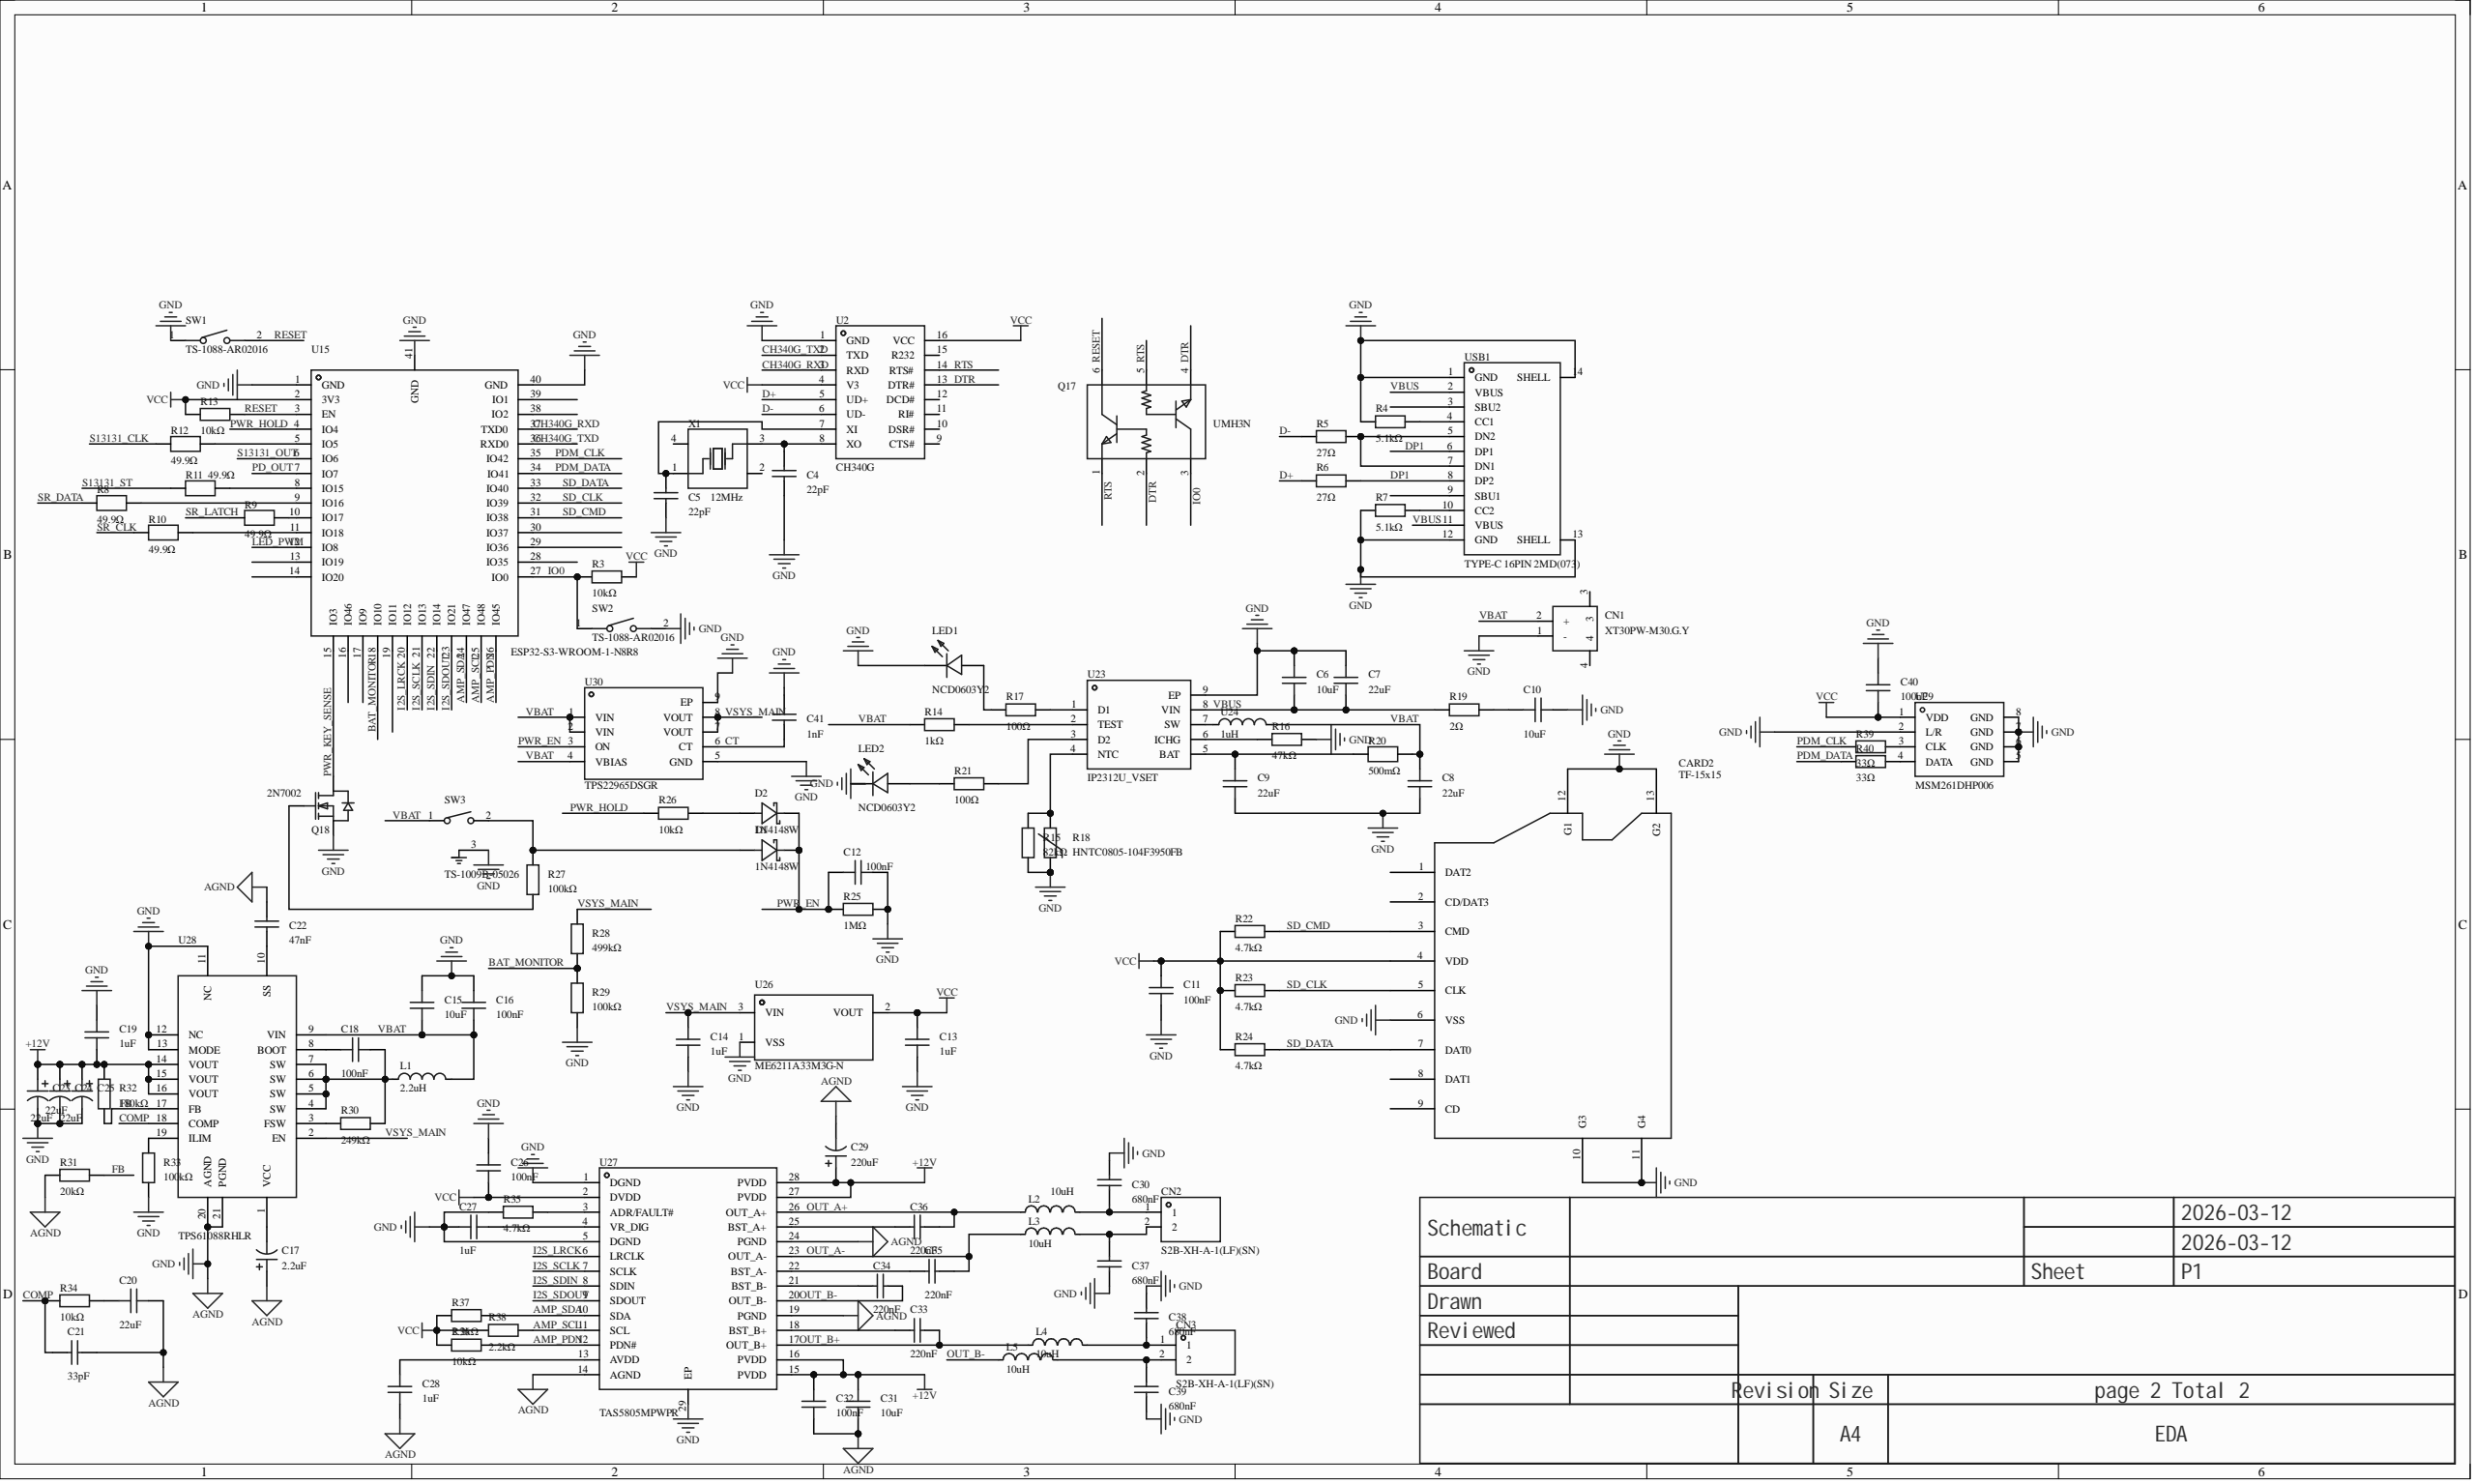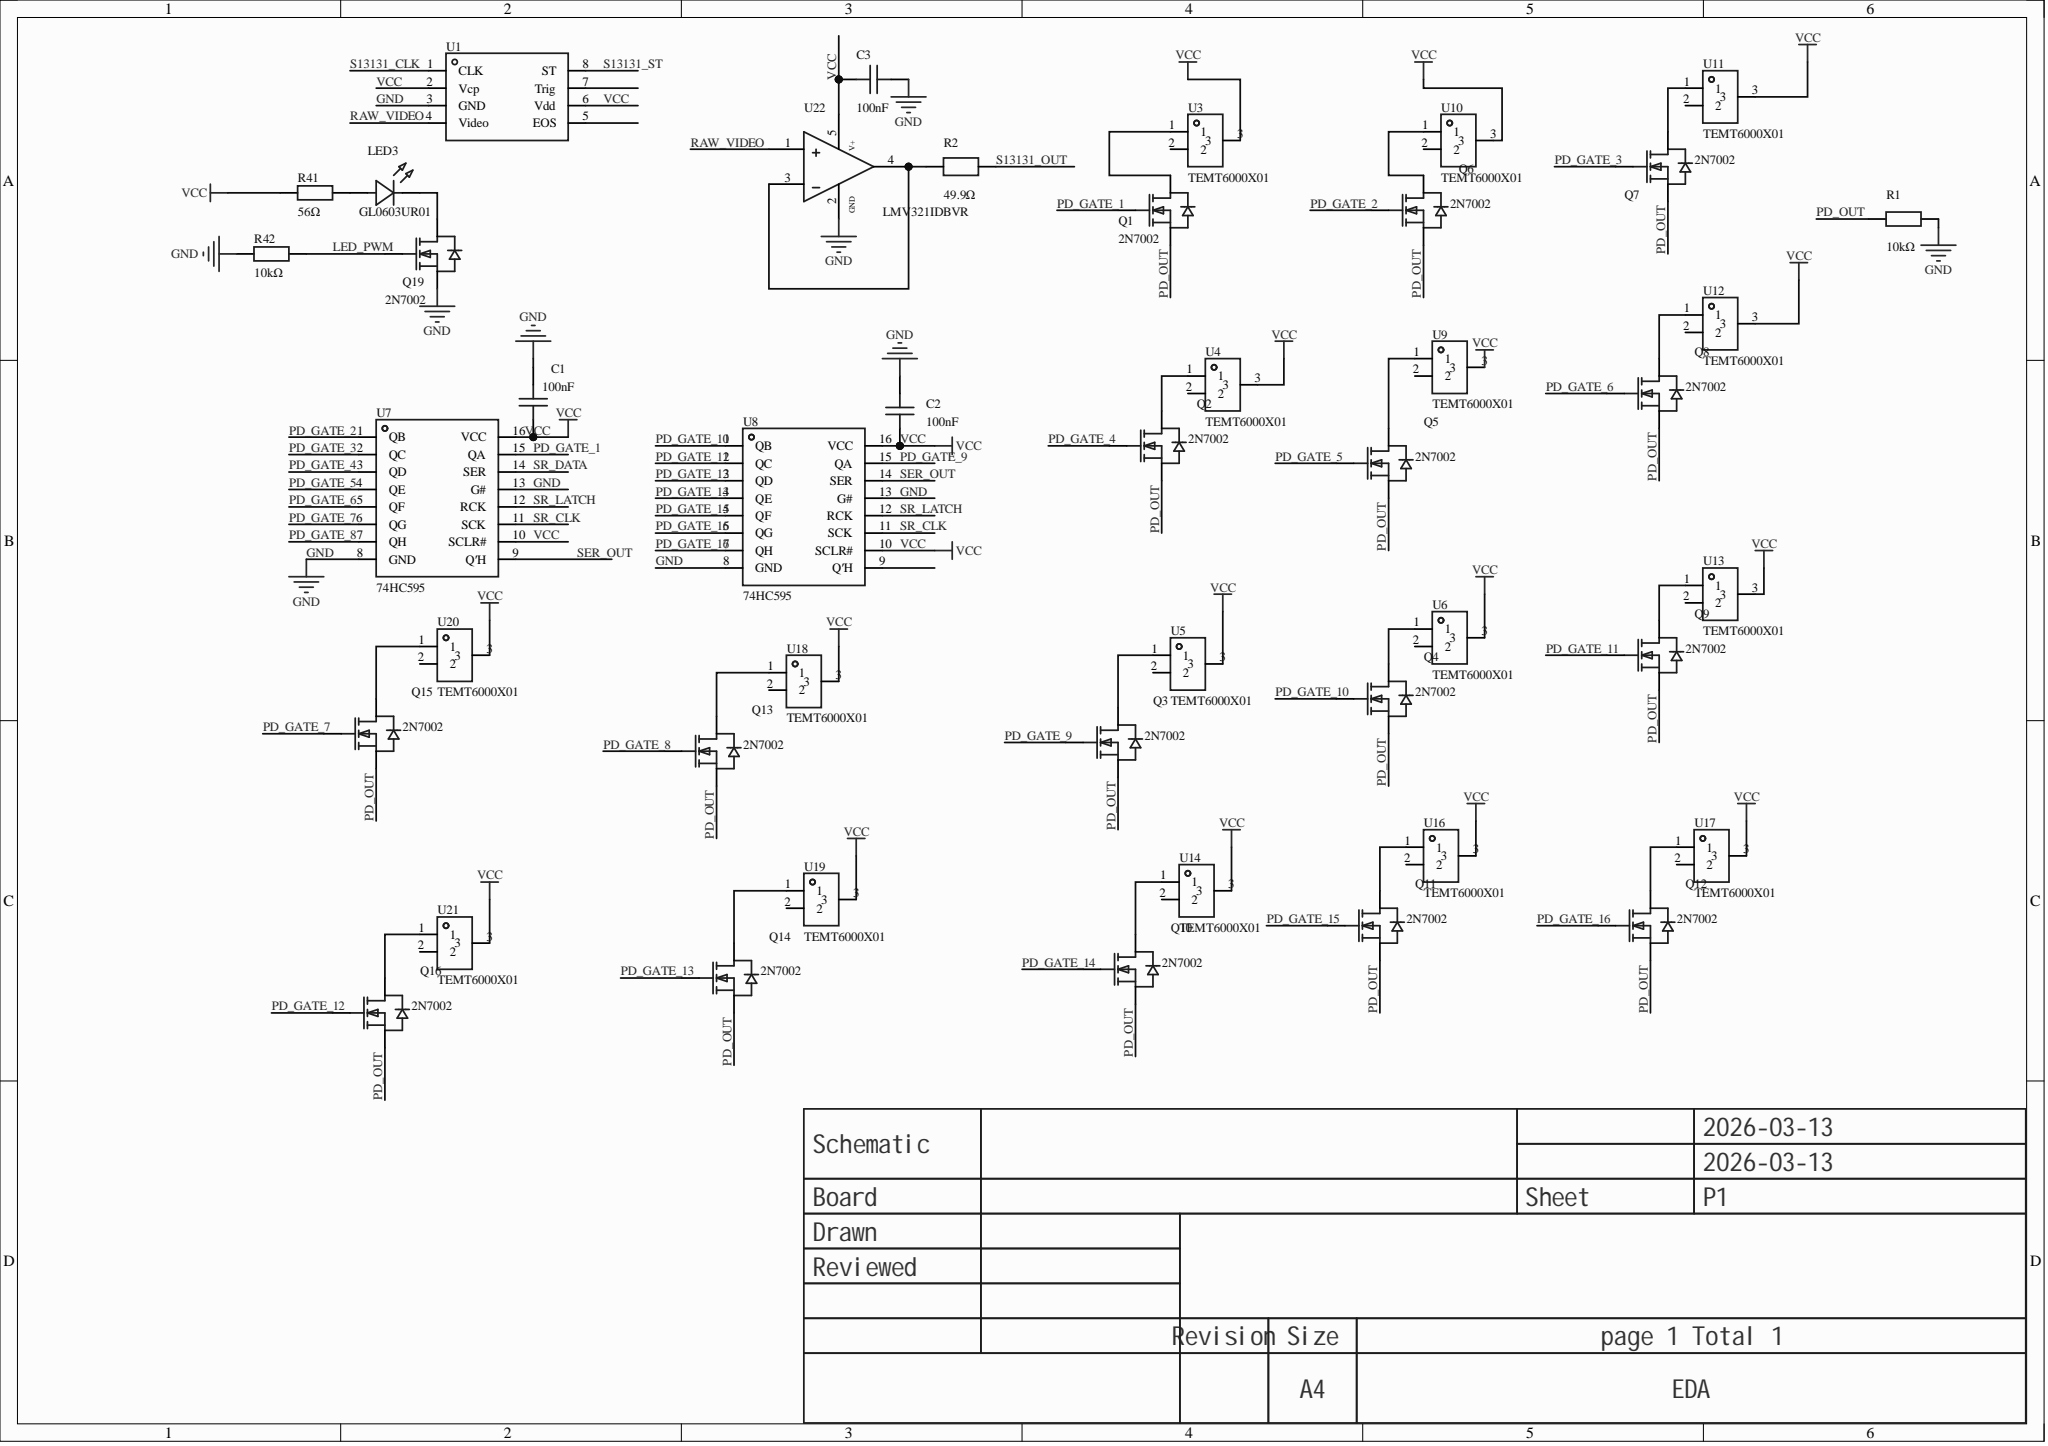Circuit board | Altium Designer | 150 parts | 126 nets
Bill of materials:
Comment,Description,Designator,Footprint,LibRef,Quantity
"100nF","Capacitance: 100nF; Tolerance: ±10%; Rated voltage: 50V; Temp. coefficient: X7R;","C1, C2, C3, C11, C12, C16, C18, C26, C32, C40","C0603","CGA0603X7R104K500JT","10"
"22pF","Capacitance: 22pF; Tolerance: ±5%; Rated voltage: 50V; Temp. coefficient: C0G;","C4, C5","C0603","CL10C220JB8NNNC","2"
"10uF","Capacitance: 10uF; Tolerance: ±20%; Rated voltage: 25V; Temp. coefficient: X5R;","C6, C10, C15, C31","C0603","CL10A106MA8NRNC","4"
"22uF","Capacitance: 22uF; Tolerance: ±20%; Rated voltage: 16V; Temp. coefficient: X5R;","C7, C8, C9, C20","C0603","CGA0603X5R226M160JT","4"
"1uF","Capacitance: 1uF; Tolerance: ±10%; Rated voltage: 50V; Temp. coefficient: X5R;","C13, C14, C19, C27, C28","C0603","CL10A105KB8NNNC","5"
"2.2uF","Capacitance: 2.2uF; Tolerance: ±20%; Rated voltage: 50V; Type: Polymer;","C17","CAP-SMD_BD5.0-L5.3-W5.3-LS6.0-FD","RYHV50V2.2UF5*5","1"
"33pF","Capacitance: 33pF; Tolerance: ±5%; Rated voltage: 50V; Temp. coefficient: C0G;","C21","C0603","CL10C330JB8NNNC","1"
"47nF","Capacitance: 47nF; Tolerance: ±10%; Rated voltage: 50V; Temp. coefficient: X7R;","C22","C0603","CL10B473KB8NNNC","1"
"22uF","Capacitance: 22uF; Tolerance: ±20%; Rated voltage: 25V; Ripple current: 26mA@120Hz;","C23, C24, C25","CAP-SMD_BD5.0-L5.3-W5.3-LS6.3-FD-1","RVT25V22M5X5","3"
"220uF","Capacitance: 220uF; Tolerance: ±20%; Rated voltage: 25V; Ripple current: 120mA@120Hz;","C29","CAP-SMD_BD6.3-L6.6-W6.6-LS7.3-FD-H7.7","JVJ25V220M6x8","1"
"680nF","Capacitance: 680nF; Tolerance: ±10%; Rated voltage: 16V; Temp. coefficient: X7R;","C30, C37, C38, C39","C0603","CC0603KRX7R7BB684","4"
"220nF","Capacitance: 220nF; Tolerance: ±10%; Rated voltage: 25V; Temp. coefficient: X7R;","C33, C34, C35, C36","C0603","CL10B224KA8NNNC","4"
"1nF","Capacitance: 1nF; Tolerance: ±10%; Rated voltage: 50V; Temp. coefficient: X7R;","C41","C0603","CL10B102KB8NNNC","1"
"TF-15x15","Card connection: Self-ejecting; Card type: MicroSD card (TF card); Connector type: Socket; Max body height: 2mm; Operating temp.: -25℃~+85℃;","CARD2","TF-SMD_TF-15-15","TF-15x15","1"
"XT30PW-M30.G.Y","Socket,DCsupply,XT30,male,PIN:2","CN1","CONN-TH_XT30PW-M","XT30PW-M30.G.Y","1"
"S2B-XH-A-1(LF)(SN)","Pin structure: 1x2P; Pitch: 2.5mm; Mounting: Right-angle THT; Series: XH; Total pins: 2P; Rows: 1; Pins per row: 2; Row spacing: -; Rated current: 3A; Contact material: Brass; Contact plating: Tin; Operating temp.: -25℃~+85℃;","CN2, CN3","CONN-TH_S2B-XH-A-1-LF-SN","S2B-XH-A-1(LF)(SN)","2"
"1N4148W","Diode configuration: Discrete; Forward voltage drop (Vf): 1.25V@150mA; DC reverse voltage (Vr): 100V; Rectified current: 150mA; Reverse recovery time (Trr): 4ns;","D1, D2","SOD-123_L2.7-W1.6-LS3.7-FD","1N4148W_C7420318","2"
"2.2uH","Inductance: 2.2uH; Tolerance: ±20%; Rated current: 4A; Saturation current (Isat): 5A; Type: Molded inductor;","L1","IND-SMD_L4.6-W4.1_MHCI04015","SRG0420-2R2-M","1"
"10uH","Inductance: 10uH; Tolerance: ±20%; Rated current: 4.5A; Saturation current (Isat): 5.5A; Type: Molded inductor;","L2, L3, L4, L5","IND-SMD_L7.3-W6.8","FXL0630-100-M","4"
"NCD0603Y2","Emitted color: Yellow; Forward voltage (VF): 1.6V~2.6V; Power: 65mW; Forward current: 20mA; Dominant wavelength: 586nm~595nm; Lens color: Clear lens; Luminous intensity: 100mcd~220mcd; Viewing angle: 130°; Operating temp.: -30℃~+85℃;","LED1, LED2","LED0603-RD","NCD0603Y2","2"
"GL0603UR01","Emitted color: Red; Forward voltage (Vf): 2.4V; Forward current: 20mA; Wavelength: 620nm~625nm; Diode configuration: Discrete diode; Lens color: Clear lens; Luminous intensity: 120mcd; Viewing angle: 120°; Tape mount: Top SMD; Operating temp.: -40℃~+85℃;","LED3","LED0603-FD","GL0603UR01","1"
"2N7002","Quantity: 1 N-channel; Drain-source voltage (Vdss): 60V; Continuous drain current (Id): 115mA; On-resistance (RDS(on)): 5Ω@10V; Power dissipation (Pd): 225mW; Threshold voltage (Vgs(th)): 2.5V;","Q1, Q2, Q3, Q4, Q5, Q6, Q7, Q8, Q9, Q10, Q11, Q12, Q13, Q14, Q15, Q16, Q18, Q19","SOT-23-3_L2.9-W1.3-P1.90-LS2.4-BR","2N7002_C8545","18"
"UMH3N","Quantity: -; Collector-emitter breakdown voltage (Vceo): 50V; Collector current (Ic): 100mA; Power dissipation (Pd): 150mW; DC current gain (hFE): 100@1mA,5V;","Q17","SC-70-6_L2.2-W1.3-P0.65-LS2.1-BR","UMH3N","1"
"10kΩ","Resistor type: Thick-film; Resistance: 10kΩ; Tolerance: ±1%; Power: 100mW; Working voltage: 75V; Temp. coefficient: ±100ppm/?;","R1, R3, R13, R26, R34, R36, R42","R0603","0603WAF1002T5E","7"
"49.9Ω","Resistor type: Thick-film; Resistance: 49.9Ω; Tolerance: ±1%; Power: 100mW; Working voltage: 75V; Temp. coefficient: ±100ppm/?;","R2, R8, R9, R10, R11, R12","R0603","FRC0603F49R9TS","6"
"5.1kΩ","Resistor type: Thick-film; Resistance: 5.1kΩ; Tolerance: ±1%; Power: 100mW; Working voltage: 75V; Temp. coefficient: ±100ppm/?;","R4, R7","R0603","0603WAF5101T5E","2"
"27Ω","Resistor type: Thick-film; Resistance: 27Ω; Tolerance: ±1%; Power: 100mW; Working voltage: 75V; Temp. coefficient: ±200ppm/?;","R5, R6","R0603","0603WAF270JT5E","2"
"1kΩ","Resistor type: Thick-film; Resistance: 1kΩ; Tolerance: ±1%; Power: 100mW; Working voltage: 75V; Temp. coefficient: ±100ppm/?;","R14","R0603","0603WAF1001T5E","1"
"82kΩ","Resistor type: Thick-film; Resistance: 82kΩ; Tolerance: ±1%; Power: 100mW; Working voltage: 75V; Temp. coefficient: ±100ppm/?;","R15","R0603","0603WAF8202T5E","1"
"47kΩ","Resistor type: Thick-film; Resistance: 47kΩ; Tolerance: ±1%; Power: 100mW; Working voltage: 75V; Temp. coefficient: ±100ppm/?;","R16","R0603","0603WAF4702T5E","1"
"100Ω","Resistor type: Thick-film; Resistance: 100Ω; Tolerance: ±1%; Power: 100mW; Max working voltage: 75V; Temp. coefficient: ±200ppm/?;","R17, R21","R0603","0603WAF1000T5E","2"
"HNTC0805-104F3950FB","","R18","R0805","HNTC0805-104F3950FB","1"
"2Ω","Resistor type: Thick-film; Resistance: 2Ω; Tolerance: ±1%; Power: 100mW; Max working voltage: 75V; Temp. coefficient: ±200ppm/?;","R19","R0603","RC0603FR-072RL","1"
"500mΩ","Resistor type: Thin-film; Resistance: 500mΩ; Tolerance: ±1%; Power: 1W; Temp. coefficient: ±100ppm/?;","R20","R1206","HoJLRH1206-1W-500mR-1%","1"
"4.7kΩ","Resistor type: Thick-film; Resistance: 4.7kΩ; Tolerance: ±1%; Power: 100mW; Working voltage: 75V; Temp. coefficient: ±100ppm/?;","R22, R23, R24, R35","R0603","0603WAF4701T5E","4"
"1MΩ","Resistor type: Thick-film; Resistance: 1MΩ; Tolerance: ±1%; Power: 100mW; Max working voltage: 75V; Temp. coefficient: ±100ppm/?;","R25","R0603","0603WAF1004T5E","1"
"100kΩ","Resistor type: Thick-film; Resistance: 100kΩ; Tolerance: ±1%; Power: 100mW; Working voltage: 75V; Temp. coefficient: ±100ppm/?;","R27, R29, R33","R0603","0603WAF1003T5E","3"
"499kΩ","Resistor type: Thick-film; Resistance: 499kΩ; Tolerance: ±1%; Power: 100mW; Working voltage: 75V; Temp. coefficient: ±100ppm/?;","R28","R0603","0603WAF4993T5E","1"
"249kΩ","Resistor type: Thick-film; Resistance: 249kΩ; Tolerance: ±1%; Power: 100mW; Working voltage: 75V; Temp. coefficient: ±100ppm/?;","R30","R0603","0603WAF2493T5E","1"
"20kΩ","Resistor type: Thick-film; Resistance: 20kΩ; Tolerance: ±1%; Power: 100mW; Working voltage: 75V; Temp. coefficient: ±100ppm/?;","R31","R0603","0603WAF2002T5E","1"
"180kΩ","Resistor type: Thick-film; Resistance: 180kΩ; Tolerance: ±1%; Power: 100mW; Working voltage: 75V; Temp. coefficient: ±100ppm/?;","R32","R0603","0603WAF1803T5E","1"
"2.2kΩ","Resistor type: Thick-film; Resistance: 2.2kΩ; Tolerance: ±1%; Power: 100mW; Max working voltage: 75V; Temp. coefficient: ±100ppm/?;","R37, R38","R0603","0603WAF2201T5E","2"
"33Ω","Resistor type: Thick-film; Resistance: 33Ω; Tolerance: ±1%; Power: 100mW; Working voltage: 75V; Temp. coefficient: ±100ppm/?;","R39, R40","R0603","0603WAF330JT5E","2"
"56Ω","Resistor type: Thick-film; Resistance: 56Ω; Tolerance: ±1%; Power: 100mW; Max working voltage: 75V; Temp. coefficient: ±200ppm/?;","R41","R0603","0603WAF560JT5E","1"
"TS-1088-AR02016","Circuit: SPST; Button shape: Round; Actuating force: 1.6N; Mounting: Upright SMD; Switch length: 4mm; Switch width: 3mm; Switch height: 2mm; Bracket: Without bracket; Contact current: 50mA; Rated voltage: 12V; Life: 10万 cycles;","SW1, SW2","SW-SMD_L3.9-W3.0-P4.45","TS-1088-AR02016","2"
"TS-1009B-05026","Circuit: SPST; Button shape: Round; Mounting: Right-angle THT; Switch length: 4.5mm; Switch width: 4.5mm; Switch height: 5mm; Contact current: 50mA; Rated voltage: 12V; LED: -; Life: -;","SW3","SW-TH_3P-L4.5-W3.8-P3.10-LS1.9_TS-1009B-05026","TS-1009B-05026","1"
"S13131-1536","","U1","BGA-8_L9.1-W2.4_S13131-1536","S13131-1536","1"
"CH340G","Application: USB to UART; Interface protocol: USB 2.0; Data rate: 2Mbps;","U2","SOIC-16_L9.9-W3.9-P1.27-LS6.0-BL","CH340G","1"
"TEMT6000X01","","U3, U4, U5, U6, U9, U10, U11, U12, U13, U14, U16, U17, U18, U19, U20, U21","SENSORS-SMD_TEMT6000X01","TEMT6000X01","16"
"74HC595","Function: Serial to serial or parallel; Working voltage: 2V~6V; Clock frequency (fc): 10MHz; Elements: 1; Bits per element: 8;","U7, U8","SOP-16_L9.9-W3.9-P1.27-LS6.0-BL","74HC595","2"
"ESP32-S3-WROOM-1-N8R8","","U15","WIRELM-SMD_ESP32-S3-WROOM-1","ESP32-S3-WROOM-1-N8R8","1"
"LMV321IDBVR","Amplifiers: Single; Rail-to-rail: Rail-to-rail output; Gain-bandwidth product (GBP): 1MHz; Input offset voltage (Vos): 7mV; Slew rate (SR): 1V/us; Input bias current (Ib): 11nA;","U22","SOT-23-5_L3.0-W1.7-P0.95-LS2.8-BR","LMV321IDBVR_C7972","1"
"IP2312U_VSET","Working voltage: 4.5V~5.5V; Max charge current: 3A; Battery type: -; Battery cells: 1;","U23","SOP-8_L4.9-W3.9-P1.27-LS6.0-BL-EP","IP2312U_VSET","1"
"1uH","Inductance: 1uH; Tolerance: ±20%; Rated current: 4A; Saturation current (Isat): 5.6A; Type: -;","U24","IND-SMD_L2.5-W2.0-VLS252012CX-150M","FTC252012S1R0MBCA","1"
"ME6211A33M3G-N","Output type: Fixed; Working voltage: 6V; Output voltage: 3.3V; Output current: 500mA; PSRR: 70dB@(1kHz); Output polarity: Positive;","U26","SOT-23-3_L2.9-W1.6-P1.90-LS2.8-BR","ME6211A33M3G-N","1"
"TAS5805MPWPR","Amplifier type: Class-D; Speaker channels: Stereo; Output power: 23W×2@8Ω; Quiescent current (Iq): 16.5mA;","U27","HTSSOP-28_L9.7-W4.4-P0.65-LS6.4-BL-EP","TAS5805MPWPR","1"
"TPS61088RHLR","Function type: Boost; Output type: Adjustable; Working voltage: 2.7V~12V; Output voltage: 4.5V~12.6V; Output current: 10A;","U28","VQFN-20_L4.6-W3.6-P0.50-BL","TPS61088RHLR","1"
"MSM261DHP006","","U29","QFN-8_L4.0-W3.0_WMM7040DTHN0-8-TR","MSM261DHP006","1"
"TPS22965DSGR","Type: Load switch; Channels: 1; Input control logic: Active high; Max continuous current: 6A; Working voltage: 800mV~5.7V; On-resistance: 16mΩ;","U30","UDFN-8_L2.0-W2.0-P0.50-TL-EP","TPS22965DSGR","1"
"TYPE-C 16PIN 2MD(073)","Connector type: Type-C; Protocol standard: -; Gender: Female; Mounting: Horizontal SMD; Contacts: 16P; Ports: 1; Rated current - power: 3A; Operating temp.: -25℃~+85℃;","USB1","USB-C-SMD_TYPE-C-6PIN-2MD-073","TYPE-C 16PIN 2MD(073)","1"
"12MHz","Crystal type: SMD crystal; Frequency: 12MHz; Room-temp. frequency deviation: ±10ppm; Load capacitance: 20pF; Frequency stability: ±20ppm;","X1","CRYSTAL-SMD_4P-L3.2-W2.5-BL","X322512MSB4SI","1"
Netlist (Protel format):
[
C1
C0603
100nF



]
[
C2
C0603
100nF



]
[
C3
C0603
100nF



]
[
C4
C0603
22pF



]
[
C5
C0603
22pF



]
[
C6
C0603
10uF



]
[
C7
C0603
22uF



]
[
C8
C0603
22uF



]
[
C9
C0603
22uF



]
[
C10
C0603
10uF



]
[
C11
C0603
100nF



]
[
C12
C0603
100nF



]
[
C13
C0603
1uF



]
[
C14
C0603
1uF



]
[
C15
C0603
10uF



]
[
C16
C0603
100nF



]
[
C17
CAP-SMD_BD5.0-L5.3-W5.3-LS6.0-FD
2.2uF



]
[
C18
C0603
100nF



]
[
C19
C0603
1uF



]
[
C20
C0603
22uF



]
[
C21
C0603
33pF



]
[
C22
C0603
47nF



]
[
C23
CAP-SMD_BD5.0-L5.3-W5.3-LS6.3-FD-1
22uF



]
[
C24
CAP-SMD_BD5.0-L5.3-W5.3-LS6.3-FD-1
22uF



]
[
C25
CAP-SMD_BD5.0-L5.3-W5.3-LS6.3-FD-1
22uF



]
[
C26
C0603
100nF



]
[
C27
C0603
1uF



]
[
C28
C0603
1uF



]
[
C29
CAP-SMD_BD6.3-L6.6-W6.6-LS7.3-FD-H7.7
220uF



]
[
C30
C0603
680nF



]
[
C31
C0603
10uF



]
[
C32
C0603
100nF



]
[
C33
C0603
220nF



]
[
C34
C0603
220nF



]
[
C35
C0603
220nF



]
[
C36
C0603
220nF



]
[
C37
C0603
680nF



]
[
C38
C0603
680nF



]
[
C39
C0603
680nF



]
[
C40
C0603
100nF



]
[
C41
C0603
1nF



]
[
CARD2
TF-SMD_TF-15-15
TF-15x15



]
[
CN1
CONN-TH_XT30PW-M
XT30PW-M30.G.Y



]
[
CN2
CONN-TH_S2B-XH-A-1-LF-SN
S2B-XH-A-1(LF)(SN)



]
[
CN3
CONN-TH_S2B-XH-A-1-LF-SN
S2B-XH-A-1(LF)(SN)



]
[
D1
SOD-123_L2.7-W1.6-LS3.7-FD
1N4148W



]
[
D2
SOD-123_L2.7-W1.6-LS3.7-FD
1N4148W



]
[
L1
IND-SMD_L4.6-W4.1_MHCI04015
2.2uH



]
[
L2
IND-SMD_L7.3-W6.8
10uH



]
[
L3
IND-SMD_L7.3-W6.8
10uH



]
[
L4
IND-SMD_L7.3-W6.8
10uH



]
[
L5
IND-SMD_L7.3-W6.8
10uH



]
[
LED1
LED0603-RD
NCD0603Y2



]
[
LED2
LED0603-RD
NCD0603Y2



]
[
LED3
LED0603-FD
GL0603UR01



]
[
Q1
SOT-23-3_L2.9-W1.3-P1.90-LS2.4-BR
2N7002



]
[
Q2
SOT-23-3_L2.9-W1.3-P1.90-LS2.4-BR
2N7002



]
[
Q3
SOT-23-3_L2.9-W1.3-P1.90-LS2.4-BR
2N7002



]
[
Q4
SOT-23-3_L2.9-W1.3-P1.90-LS2.4-BR
2N7002



]
[
Q5
SOT-23-3_L2.9-W1.3-P1.90-LS2.4-BR
2N7002



]
[
Q6
SOT-23-3_L2.9-W1.3-P1.90-LS2.4-BR
2N7002



]
[
Q7
SOT-23-3_L2.9-W1.3-P1.90-LS2.4-BR
2N7002



]
[
Q8
SOT-23-3_L2.9-W1.3-P1.90-LS2.4-BR
2N7002



]
[
Q9
SOT-23-3_L2.9-W1.3-P1.90-LS2.4-BR
2N7002



]
[
Q10
SOT-23-3_L2.9-W1.3-P1.90-LS2.4-BR
2N7002



]
[
Q11
SOT-23-3_L2.9-W1.3-P1.90-LS2.4-BR
2N7002



]
[
Q12
SOT-23-3_L2.9-W1.3-P1.90-LS2.4-BR
2N7002



]
[
Q13
SOT-23-3_L2.9-W1.3-P1.90-LS2.4-BR
2N7002



]
[
Q14
SOT-23-3_L2.9-W1.3-P1.90-LS2.4-BR
2N7002



]
[
Q15
SOT-23-3_L2.9-W1.3-P1.90-LS2.4-BR
2N7002



]
[
Q16
SOT-23-3_L2.9-W1.3-P1.90-LS2.4-BR
2N7002



]
[
Q17
SC-70-6_L2.2-W1.3-P0.65-LS2.1-BR
UMH3N



]
[
Q18
SOT-23-3_L2.9-W1.3-P1.90-LS2.4-BR
2N7002



]
[
Q19
SOT-23-3_L2.9-W1.3-P1.90-LS2.4-BR
2N7002



]
[
R1
R0603
10kΩ



]
[
R2
R0603
49.9Ω



]
[
R3
R0603
10kΩ



]
[
R4
R0603
5.1kΩ



]
[
R5
R0603
27Ω



]
[
R6
R0603
27Ω



]
[
R7
R0603
5.1kΩ



]
[
R8
R0603
49.9Ω



]
[
R9
R0603
49.9Ω



]
[
R10
R0603
49.9Ω



]
[
R11
R0603
49.9Ω



]
[
R12
R0603
49.9Ω



]
[
R13
R0603
10kΩ



]
[
R14
R0603
1kΩ



]
[
R15
R0603
82kΩ



]
[
R16
R0603
47kΩ



]
[
R17
R0603
100Ω



]
[
R18
R0805
HNTC0805-104F3950FB



]
[
R19
R0603
2Ω



]
[
R20
R1206
500mΩ



]
[
R21
R0603
100Ω



]
[
R22
R0603
4.7kΩ



]
[
R23
R0603
4.7kΩ



]
[
R24
R0603
4.7kΩ



]
[
R25
R0603
1MΩ



]
[
R26
R0603
10kΩ



]
[
R27
R0603
100kΩ



]
[
R28
R0603
499kΩ



]
[
R29
R0603
100kΩ



]
[
R30
R0603
249kΩ



]
[
R31
R0603
20kΩ



]
[
R32
R0603
180kΩ



]
[
R33
R0603
100kΩ



]
[
R34
R0603
10kΩ



]
[
R35
R0603
4.7kΩ



]
[
R36
R0603
10kΩ



]
[
R37
R0603
2.2kΩ



]
[
R38
R0603
2.2kΩ



]
[
R39
R0603
33Ω



]
[
R40
R0603
33Ω



]
[
R41
R0603
56Ω



]
[
R42
R0603
10kΩ



]
[
SW1
SW-SMD_L3.9-W3.0-P4.45
TS-1088-AR02016



]
[
SW2
SW-SMD_L3.9-W3.0-P4.45
TS-1088-AR02016



]
[
SW3
SW-TH_3P-L4.5-W3.8-P3.10-LS1.9_TS-1009B-05026
TS-1009B-05026



]
[
U1
BGA-8_L9.1-W2.4_S13131-1536
S13131-1536



]
[
U2
SOIC-16_L9.9-W3.9-P1.27-LS6.0-BL
CH340G



]
[
U3
SENSORS-SMD_TEMT6000X01
TEMT6000X01



]
[
U4
SENSORS-SMD_TEMT6000X01
TEMT6000X01



]
[
U5
SENSORS-SMD_TEMT6000X01
TEMT6000X01



]
[
U6
SENSORS-SMD_TEMT6000X01
TEMT6000X01



]
[
U7
SOP-16_L9.9-W3.9-P1.27-LS6.0-BL
74HC595



]
[
U8
SOP-16_L9.9-W3.9-P1.27-LS6.0-BL
74HC595



]
[
U9
SENSORS-SMD_TEMT6000X01
TEMT6000X01



]
[
U10
SENSORS-SMD_TEMT6000X01
TEMT6000X01



]
[
U11
SENSORS-SMD_TEMT6000X01
TEMT6000X01



]
[
U12
SENSORS-SMD_TEMT6000X01
TEMT6000X01



]
[
U13
SENSORS-SMD_TEMT6000X01
TEMT6000X01



]
[
U14
SENSORS-SMD_TEMT6000X01
TEMT6000X01



]
[
U15
WIRELM-SMD_ESP32-S3-WROOM-1
ESP32-S3-WROOM-1-N8R8



]
[
U16
SENSORS-SMD_TEMT6000X01
TEMT6000X01



]
[
U17
SENSORS-SMD_TEMT6000X01
TEMT6000X01



]
[
U18
SENSORS-SMD_TEMT6000X01
TEMT6000X01



]
[
U19
SENSORS-SMD_TEMT6000X01
TEMT6000X01



]
[
U20
SENSORS-SMD_TEMT6000X01
TEMT6000X01



]
[
U21
SENSORS-SMD_TEMT6000X01
TEMT6000X01



]
[
U22
SOT-23-5_L3.0-W1.7-P0.95-LS2.8-BR
LMV321IDBVR



]
[
U23
SOP-8_L4.9-W3.9-P1.27-LS6.0-BL-EP
IP2312U_VSET



]
[
U24
IND-SMD_L2.5-W2.0-VLS252012CX-150M
1uH



]
[
U26
SOT-23-3_L2.9-W1.6-P1.90-LS2.8-BR
ME6211A33M3G-N



]
[
U27
HTSSOP-28_L9.7-W4.4-P0.65-LS6.4-BL-EP
TAS5805MPWPR



]
[
U28
VQFN-20_L4.6-W3.6-P0.50-BL
TPS61088RHLR



]
[
U29
QFN-8_L4.0-W3.0_WMM7040DTHN0-8-TR
MSM261DHP006



]
[
U30
UDFN-8_L2.0-W2.0-P0.50-TL-EP
TPS22965DSGR



]
[
USB1
USB-C-SMD_TYPE-C-6PIN-2MD-073
TYPE-C 16PIN 2MD(073)



]
[
X1
CRYSTAL-SMD_4P-L3.2-W2.5-BL
12MHz



]
(
VSYS_MAIN
C14-2
R28-2
U26-3
U28-2
U30-7
U30-8
)
(
VCC
C1-1
C2-1
C3-1
C11-2
C13-2
C26-1
C40-1
CARD2-4
R3-2
R13-1
R22-1
R23-1
R24-1
R36-1
R37-1
R38-1
R41-1
U1-2
U1-6
U2-4
U2-16
U3-3
U4-3
U5-3
U6-3
U7-10
U7-16
U8-10
U8-16
U9-3
U10-3
U11-3
U12-3
U13-3
U14-3
U15-2
U16-3
U17-3
U18-3
U19-3
U20-3
U21-3
U22-5
U26-2
U27-2
U29-1
)
(
VBUS
C6-1
C7-1
R19-1
U23-8
USB1-2
USB1-11
)
(
VBAT
C8-2
C15-1
C16-1
CN1-2
L1-2
R14-1
R20-2
SW3-1
U24-2
U28-9
U30-1
U30-2
U30-4
)
(
SR_LATCH
R9-2
U7-12
U8-12
)
(
SR_DATA
R8-2
U7-14
)
(
SR_CLK
R10-1
U7-11
U8-11
)
(
SER_OUT
U7-9
U8-14
)
(
SD_DATA
CARD2-7
R24-2
U15-33
)
(
SD_CMD
CARD2-3
R22-2
U15-31
)
(
SD_CLK
CARD2-5
R23-2
U15-32
)
(
S13131_ST
R11-1
U1-8
)
(
S13131_OUT
R2-2
U15-6
)
(
S13131_CLK
R12-1
U1-1
)
(
RTS
Q17-1
Q17-5
U2-14
)
(
RESET
Q17-6
R13-2
SW1-2
U15-3
)
(
RAW_VIDEO
U1-4
U22-1
)
(
PWR_KEY_SENSE
Q18-3
U15-15
)
(
PWR_HOLD
R26-1
U15-4
)
(
PWR_EN
C12-1
D1-2
D2-2
R25-1
U30-3
)
(
PDM_DATA
R40-1
U15-34
)
(
PDM_CLK
R39-1
U15-35
)
(
PD_OUT
Q1-2
Q2-2
Q3-2
Q4-2
Q5-2
Q6-2
Q7-2
Q8-2
Q9-2
Q10-2
Q11-2
Q12-2
Q13-2
Q14-2
Q15-2
Q16-2
R1-1
U15-7
)
(
PD_GATE_16
Q12-1
U8-7
)
(
PD_GATE_15
Q11-1
U8-6
)
(
PD_GATE_14
Q10-1
U8-5
)
(
PD_GATE_13
Q14-1
U8-4
)
(
PD_GATE_12
Q16-1
U8-3
)
(
PD_GATE_11
Q9-1
U8-2
)
(
PD_GATE_10
Q4-1
U8-1
)
(
PD_GATE_9
Q3-1
U8-15
)
(
PD_GATE_8
Q13-1
U7-7
)
(
PD_GATE_7
Q15-1
U7-6
)
(
PD_GATE_6
Q8-1
U7-5
)
(
PD_GATE_5
Q5-1
U7-4
)
(
PD_GATE_4
Q2-1
U7-3
)
(
PD_GATE_3
Q7-1
U7-2
)
(
PD_GATE_2
Q6-1
U7-1
)
(
PD_GATE_1
Q1-1
U7-15
)
(
OUT_B-
C34-2
L5-1
U27-20
)
(
OUT_B+
C33-2
L4-1
U27-17
)
(
OUT_A-
C35-2
L3-1
U27-23
)
(
OUT_A+
C36-2
L2-1
U27-26
)
(
NetU23_7
U23-7
U24-1
)
(
NetR40_2
R40-2
U29-4
)
(
NetR39_2
R39-2
U29-3
)
(
NetR35_2
R35-2
U27-3
)
(
NetR33_2
R33-2
U28-19
)
(
NetR30_1
R30-1
U28-3
)
(
NetR21_2
R21-2
U23-3
)
(
NetR17_2
R17-2
U23-1
)
(
NetR16_1
R16-1
U23-6
)
(
NetR15_2
R15-2
R18-2
U23-4
)
(
NetR14_2
R14-2
U23-2
)
(
NetR12_2
R12-2
U15-5
)
(
NetR11_2
R11-2
U15-8
)
(
NetR10_2
R10-2
U15-11
)
(
NetR9_1
R9-1
U15-10
)
(
NetR8_1
R8-1
U15-9
)
(
NetR7_2
R7-2
USB1-10
)
(
NetR5_2
R5-2
USB1-5
USB1-7
)
(
NetR4_2
R4-2
USB1-4
)
(
NetR2_1
R2-1
U22-3
U22-4
)
(
NetQ18_1
Q18-1
R27-1
)
(
NetQ16_3
Q16-3
U21-1
)
(
NetQ15_3
Q15-3
U20-1
)
(
NetQ14_3
Q14-3
U19-1
)
(
NetQ13_3
Q13-3
U18-1
)
(
NetQ12_3
Q12-3
U17-1
)
(
NetQ11_3
Q11-3
U16-1
)
(
NetQ10_3
Q10-3
U14-1
)
(
NetQ9_3
Q9-3
U13-1
)
(
NetQ8_3
Q8-3
U12-1
)
(
NetQ7_3
Q7-3
U11-1
)
(
NetQ6_3
Q6-3
U10-1
)
(
NetQ5_3
Q5-3
U9-1
)
(
NetQ4_3
Q4-3
U6-1
)
(
NetQ3_3
Q3-3
U5-1
)
(
NetQ2_3
Q2-3
U4-1
)
(
NetQ1_3
Q1-3
U3-1
)
(
NetLED3_2
LED3-2
Q19-3
)
(
NetLED3_1
LED3-1
R41-2
)
(
NetLED2_2
LED2-2
R21-1
)
(
NetLED1_2
LED1-2
R17-1
)
(
NetD2_1
D2-1
R26-2
)
(
NetD1_1
D1-1
R27-2
SW3-2
)
(
NetC39_2
C39-2
CN3-2
L5-2
)
(
NetC38_1
C38-1
CN3-1
L4-2
)
(
NetC37_2
C37-2
CN2-2
L3-2
)
(
NetC36_1
C36-1
U27-25
)
(
NetC35_1
C35-1
U27-22
)
(
NetC34_1
C34-1
U27-21
)
(
NetC33_1
C33-1
U27-18
)
(
NetC30_1
C30-1
CN2-1
L2-2
)
(
NetC28_2
C28-2
U27-13
)
(
NetC27_1
C27-1
U27-4
)
(
NetC22_1
C22-1
U28-10
)
(
NetC20_1
C20-1
R34-2
)
(
NetC18_2
C18-2
L1-1
R30-2
U28-4
U28-5
U28-6
U28-7
)
(
NetC18_1
C18-1
U28-8
)
(
NetC17_2
C17-2
U28-1
)
(
NetC10_1
C10-1
R19-2
)
(
NetC9_2
C9-2
R20-1
U23-5
)
(
NetC5_2
C5-2
U2-7
X1-1
)
(
NetC4_2
C4-2
U2-8
X1-3
)
(
LED_PWM
Q19-1
R42-1
U15-12
)
(
IO0
Q17-3
R3-1
SW2-1
U15-27
)
(
I2S_SDOUT
U15-23
U27-9
)
(
I2S_SDIN
U15-22
U27-8
)
(
I2S_SCLK
U15-21
U27-7
)
(
I2S_LRCK
U15-20
U27-6
)
(
GND
C1-2
C2-2
C3-2
C4-1
C5-1
C6-2
C7-2
C8-1
C9-1
C10-2
C11-1
C12-2
C13-1
C14-1
C15-2
C16-2
C17-1
C19-2
C20-2
C21-2
C22-2
C23-2
C24-2
C25-2
C26-2
C27-2
C28-1
C29-2
C30-2
C31-1
C32-1
C37-1
C38-2
C39-1
C40-2
C41-2
CARD2-6
CARD2-10
CARD2-11
CARD2-12
CARD2-13
CN1-1
LED1-1
LED2-1
Q18-2
Q19-2
R1-2
R4-1
R7-1
R15-1
R16-2
R18-1
R25-2
R29-1
R31-1
R33-1
R35-1
R42-2
SW1-1
SW2-2
SW3-3
U1-3
U2-1
U7-8
U7-13
U8-8
U8-13
U15-1
U15-40
U15-41
U22-2
U23-9
U26-1
U27-1
U27-5
U27-14
U27-19
U27-24
U27-29
U28-11
U28-12
U28-13
U28-20
U28-21
U29-2
U29-5
U29-6
U29-7
U29-8
U30-5
U30-9
USB1-1
USB1-12
USB1-13
USB1-14
)
(
FB
R31-2
R32-1
U28-17
)
(
DTR
Q17-2
Q17-4
U2-13
)
(
DP1
R6-2
USB1-6
USB1-8
)
(
D-
R5-1
U2-6
)
(
D+
R6-1
U2-5
)
(
CT
C41-1
U30-6
)
(
COMP
C21-1
R34-1
U28-18
)
(
CH340G_TXD
U2-2
U15-36
)
(
CH340G_RXD
U2-3
U15-37
)
(
BAT_MONITOR
R28-1
R29-2
U15-18
)
(
AMP_SDA
R37-2
U15-24
U27-10
)
(
AMP_SCL
R38-2
U15-25
U27-11
)
(
AMP_PDN
R36-2
U15-26
U27-12
)
(
+12V
C19-1
C23-1
C24-1
C25-1
C29-1
C31-2
C32-2
R32-2
U27-15
U27-16
U27-27
U27-28
U28-14
U28-15
U28-16
)